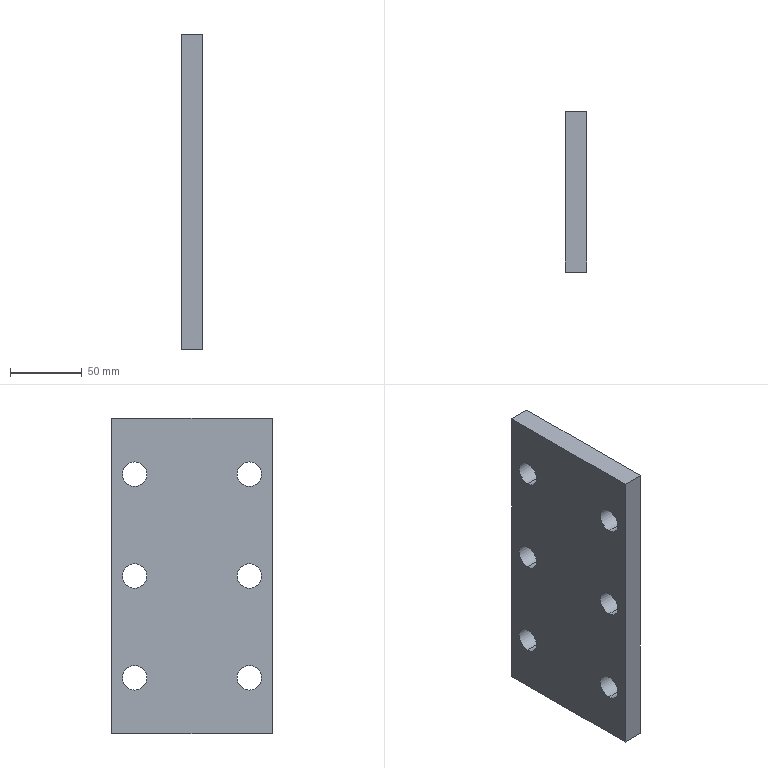Part | SolidWorks | features ICE 3, Extrusion 1 | 1 solid | 18 faces | box 15 x 112 x 220 mm | volume 349172 mm3 | cylinder 12 | plane 6 | commonest cylinder face diameters 17 x12
STEP:
#1=CARTESIAN_POINT('',(60.,-40.,101.5));
#2=VERTEX_POINT('',#1);
#3=CARTESIAN_POINT('',(60.,-40.,118.5));
#4=VERTEX_POINT('',#3);
#5=CARTESIAN_POINT('',(60.,-40.,110.));
#6=DIRECTION('',(-1.,0.,0.));
#7=DIRECTION('',(0.,1.,0.));
#8=AXIS2_PLACEMENT_3D('',#5,#6,#7);
#9=CIRCLE('',#8,8.5);
#10=EDGE_CURVE('',#2,#4,#9,.T.);
#11=ORIENTED_EDGE('',*,*,#10,.T.);
#12=CARTESIAN_POINT('',(75.,-40.,118.5));
#13=VERTEX_POINT('',#12);
#14=CARTESIAN_POINT('',(-45.001,-40.,118.5));
#15=DIRECTION('',(1.,0.,0.));
#16=VECTOR('',#15,1000.);
#17=LINE('',#14,#16);
#18=EDGE_CURVE('',#4,#13,#17,.T.);
#19=ORIENTED_EDGE('',*,*,#18,.T.);
#20=CARTESIAN_POINT('',(75.,-40.,101.5));
#21=VERTEX_POINT('',#20);
#22=CARTESIAN_POINT('',(75.,-40.,110.));
#23=DIRECTION('',(1.,0.,0.));
#24=DIRECTION('',(0.,0.,-1.));
#25=AXIS2_PLACEMENT_3D('',#22,#23,#24);
#26=CIRCLE('',#25,8.5);
#27=EDGE_CURVE('',#13,#21,#26,.T.);
#28=ORIENTED_EDGE('',*,*,#27,.T.);
#29=CARTESIAN_POINT('',(-45.001,-40.,101.5));
#30=DIRECTION('',(1.,0.,0.));
#31=VECTOR('',#30,1000.);
#32=LINE('',#29,#31);
#33=EDGE_CURVE('',#2,#21,#32,.T.);
#34=ORIENTED_EDGE('',*,*,#33,.F.);
#35=EDGE_LOOP('',(#11,#19,#28,#34));
#36=FACE_OUTER_BOUND('',#35,.T.);
#37=CARTESIAN_POINT('',(-45.001,-40.,110.));
#38=DIRECTION('',(1.,0.,0.));
#39=DIRECTION('',(0.,0.,-1.));
#40=AXIS2_PLACEMENT_3D('',#37,#38,#39);
#41=CYLINDRICAL_SURFACE('',#40,8.5);
#42=ADVANCED_FACE('',(#36),#41,.F.);
#43=CARTESIAN_POINT('',(60.,-40.,30.5));
#44=VERTEX_POINT('',#43);
#45=CARTESIAN_POINT('',(60.,-40.,47.5));
#46=VERTEX_POINT('',#45);
#47=CARTESIAN_POINT('',(60.,-40.,39.));
#48=DIRECTION('',(-1.,0.,0.));
#49=DIRECTION('',(0.,1.,0.));
#50=AXIS2_PLACEMENT_3D('',#47,#48,#49);
#51=CIRCLE('',#50,8.5);
#52=EDGE_CURVE('',#44,#46,#51,.T.);
#53=ORIENTED_EDGE('',*,*,#52,.T.);
#54=CARTESIAN_POINT('',(75.,-40.,47.5));
#55=VERTEX_POINT('',#54);
#56=CARTESIAN_POINT('',(-45.001,-40.,47.5));
#57=DIRECTION('',(1.,0.,0.));
#58=VECTOR('',#57,1000.);
#59=LINE('',#56,#58);
#60=EDGE_CURVE('',#46,#55,#59,.T.);
#61=ORIENTED_EDGE('',*,*,#60,.T.);
#62=CARTESIAN_POINT('',(75.,-40.,30.5));
#63=VERTEX_POINT('',#62);
#64=CARTESIAN_POINT('',(75.,-40.,39.));
#65=DIRECTION('',(1.,0.,0.));
#66=DIRECTION('',(0.,0.,-1.));
#67=AXIS2_PLACEMENT_3D('',#64,#65,#66);
#68=CIRCLE('',#67,8.5);
#69=EDGE_CURVE('',#55,#63,#68,.T.);
#70=ORIENTED_EDGE('',*,*,#69,.T.);
#71=CARTESIAN_POINT('',(-45.001,-40.,30.5));
#72=DIRECTION('',(1.,0.,0.));
#73=VECTOR('',#72,1000.);
#74=LINE('',#71,#73);
#75=EDGE_CURVE('',#44,#63,#74,.T.);
#76=ORIENTED_EDGE('',*,*,#75,.F.);
#77=EDGE_LOOP('',(#53,#61,#70,#76));
#78=FACE_OUTER_BOUND('',#77,.T.);
#79=CARTESIAN_POINT('',(-45.001,-40.,39.));
#80=DIRECTION('',(1.,0.,0.));
#81=DIRECTION('',(0.,0.,-1.));
#82=AXIS2_PLACEMENT_3D('',#79,#80,#81);
#83=CYLINDRICAL_SURFACE('',#82,8.5);
#84=ADVANCED_FACE('',(#78),#83,.F.);
#85=CARTESIAN_POINT('',(60.,-40.,172.5));
#86=VERTEX_POINT('',#85);
#87=CARTESIAN_POINT('',(60.,-40.,189.5));
#88=VERTEX_POINT('',#87);
#89=CARTESIAN_POINT('',(60.,-40.,181.));
#90=DIRECTION('',(-1.,0.,0.));
#91=DIRECTION('',(0.,1.,0.));
#92=AXIS2_PLACEMENT_3D('',#89,#90,#91);
#93=CIRCLE('',#92,8.5);
#94=EDGE_CURVE('',#86,#88,#93,.T.);
#95=ORIENTED_EDGE('',*,*,#94,.T.);
#96=CARTESIAN_POINT('',(75.,-40.,189.5));
#97=VERTEX_POINT('',#96);
#98=CARTESIAN_POINT('',(-45.001,-40.,189.5));
#99=DIRECTION('',(1.,0.,0.));
#100=VECTOR('',#99,1000.);
#101=LINE('',#98,#100);
#102=EDGE_CURVE('',#88,#97,#101,.T.);
#103=ORIENTED_EDGE('',*,*,#102,.T.);
#104=CARTESIAN_POINT('',(75.,-40.,172.5));
#105=VERTEX_POINT('',#104);
#106=CARTESIAN_POINT('',(75.,-40.,181.));
#107=DIRECTION('',(1.,0.,0.));
#108=DIRECTION('',(0.,0.,-1.));
#109=AXIS2_PLACEMENT_3D('',#106,#107,#108);
#110=CIRCLE('',#109,8.5);
#111=EDGE_CURVE('',#97,#105,#110,.T.);
#112=ORIENTED_EDGE('',*,*,#111,.T.);
#113=CARTESIAN_POINT('',(-45.001,-40.,172.5));
#114=DIRECTION('',(1.,0.,0.));
#115=VECTOR('',#114,1000.);
#116=LINE('',#113,#115);
#117=EDGE_CURVE('',#86,#105,#116,.T.);
#118=ORIENTED_EDGE('',*,*,#117,.F.);
#119=EDGE_LOOP('',(#95,#103,#112,#118));
#120=FACE_OUTER_BOUND('',#119,.T.);
#121=CARTESIAN_POINT('',(-45.001,-40.,181.));
#122=DIRECTION('',(1.,0.,0.));
#123=DIRECTION('',(0.,0.,-1.));
#124=AXIS2_PLACEMENT_3D('',#121,#122,#123);
#125=CYLINDRICAL_SURFACE('',#124,8.5);
#126=ADVANCED_FACE('',(#120),#125,.F.);
#127=CARTESIAN_POINT('',(60.,40.,172.5));
#128=VERTEX_POINT('',#127);
#129=CARTESIAN_POINT('',(60.,40.,189.5));
#130=VERTEX_POINT('',#129);
#131=CARTESIAN_POINT('',(60.,40.,181.));
#132=DIRECTION('',(-1.,0.,0.));
#133=DIRECTION('',(0.,1.,0.));
#134=AXIS2_PLACEMENT_3D('',#131,#132,#133);
#135=CIRCLE('',#134,8.5);
#136=EDGE_CURVE('',#128,#130,#135,.T.);
#137=ORIENTED_EDGE('',*,*,#136,.T.);
#138=CARTESIAN_POINT('',(75.,40.,189.5));
#139=VERTEX_POINT('',#138);
#140=CARTESIAN_POINT('',(-45.001,40.,189.5));
#141=DIRECTION('',(1.,0.,0.));
#142=VECTOR('',#141,1000.);
#143=LINE('',#140,#142);
#144=EDGE_CURVE('',#130,#139,#143,.T.);
#145=ORIENTED_EDGE('',*,*,#144,.T.);
#146=CARTESIAN_POINT('',(75.,40.,172.5));
#147=VERTEX_POINT('',#146);
#148=CARTESIAN_POINT('',(75.,40.,181.));
#149=DIRECTION('',(1.,0.,0.));
#150=DIRECTION('',(0.,0.,-1.));
#151=AXIS2_PLACEMENT_3D('',#148,#149,#150);
#152=CIRCLE('',#151,8.5);
#153=EDGE_CURVE('',#139,#147,#152,.T.);
#154=ORIENTED_EDGE('',*,*,#153,.T.);
#155=CARTESIAN_POINT('',(-45.001,40.,172.5));
#156=DIRECTION('',(1.,0.,0.));
#157=VECTOR('',#156,1000.);
#158=LINE('',#155,#157);
#159=EDGE_CURVE('',#128,#147,#158,.T.);
#160=ORIENTED_EDGE('',*,*,#159,.F.);
#161=EDGE_LOOP('',(#137,#145,#154,#160));
#162=FACE_OUTER_BOUND('',#161,.T.);
#163=CARTESIAN_POINT('',(-45.001,40.,181.));
#164=DIRECTION('',(1.,0.,0.));
#165=DIRECTION('',(0.,0.,-1.));
#166=AXIS2_PLACEMENT_3D('',#163,#164,#165);
#167=CYLINDRICAL_SURFACE('',#166,8.5);
#168=ADVANCED_FACE('',(#162),#167,.F.);
#169=CARTESIAN_POINT('',(60.,40.,101.5));
#170=VERTEX_POINT('',#169);
#171=CARTESIAN_POINT('',(60.,40.,118.5));
#172=VERTEX_POINT('',#171);
#173=CARTESIAN_POINT('',(60.,40.,110.));
#174=DIRECTION('',(-1.,0.,0.));
#175=DIRECTION('',(0.,1.,0.));
#176=AXIS2_PLACEMENT_3D('',#173,#174,#175);
#177=CIRCLE('',#176,8.5);
#178=EDGE_CURVE('',#170,#172,#177,.T.);
#179=ORIENTED_EDGE('',*,*,#178,.T.);
#180=CARTESIAN_POINT('',(75.,40.,118.5));
#181=VERTEX_POINT('',#180);
#182=CARTESIAN_POINT('',(-45.001,40.,118.5));
#183=DIRECTION('',(1.,0.,0.));
#184=VECTOR('',#183,1000.);
#185=LINE('',#182,#184);
#186=EDGE_CURVE('',#172,#181,#185,.T.);
#187=ORIENTED_EDGE('',*,*,#186,.T.);
#188=CARTESIAN_POINT('',(75.,40.,101.5));
#189=VERTEX_POINT('',#188);
#190=CARTESIAN_POINT('',(75.,40.,110.));
#191=DIRECTION('',(1.,0.,0.));
#192=DIRECTION('',(0.,0.,-1.));
#193=AXIS2_PLACEMENT_3D('',#190,#191,#192);
#194=CIRCLE('',#193,8.5);
#195=EDGE_CURVE('',#181,#189,#194,.T.);
#196=ORIENTED_EDGE('',*,*,#195,.T.);
#197=CARTESIAN_POINT('',(-45.001,40.,101.5));
#198=DIRECTION('',(1.,0.,0.));
#199=VECTOR('',#198,1000.);
#200=LINE('',#197,#199);
#201=EDGE_CURVE('',#170,#189,#200,.T.);
#202=ORIENTED_EDGE('',*,*,#201,.F.);
#203=EDGE_LOOP('',(#179,#187,#196,#202));
#204=FACE_OUTER_BOUND('',#203,.T.);
#205=CARTESIAN_POINT('',(-45.001,40.,110.));
#206=DIRECTION('',(1.,0.,0.));
#207=DIRECTION('',(0.,0.,-1.));
#208=AXIS2_PLACEMENT_3D('',#205,#206,#207);
#209=CYLINDRICAL_SURFACE('',#208,8.5);
#210=ADVANCED_FACE('',(#204),#209,.F.);
#211=CARTESIAN_POINT('',(60.,40.,30.5));
#212=VERTEX_POINT('',#211);
#213=CARTESIAN_POINT('',(60.,40.,47.5));
#214=VERTEX_POINT('',#213);
#215=CARTESIAN_POINT('',(60.,40.,39.));
#216=DIRECTION('',(-1.,0.,0.));
#217=DIRECTION('',(0.,1.,0.));
#218=AXIS2_PLACEMENT_3D('',#215,#216,#217);
#219=CIRCLE('',#218,8.5);
#220=EDGE_CURVE('',#212,#214,#219,.T.);
#221=ORIENTED_EDGE('',*,*,#220,.T.);
#222=CARTESIAN_POINT('',(75.,40.,47.5));
#223=VERTEX_POINT('',#222);
#224=CARTESIAN_POINT('',(-45.001,40.,47.5));
#225=DIRECTION('',(1.,0.,0.));
#226=VECTOR('',#225,1000.);
#227=LINE('',#224,#226);
#228=EDGE_CURVE('',#214,#223,#227,.T.);
#229=ORIENTED_EDGE('',*,*,#228,.T.);
#230=CARTESIAN_POINT('',(75.,40.,30.5));
#231=VERTEX_POINT('',#230);
#232=CARTESIAN_POINT('',(75.,40.,39.));
#233=DIRECTION('',(1.,0.,0.));
#234=DIRECTION('',(0.,0.,-1.));
#235=AXIS2_PLACEMENT_3D('',#232,#233,#234);
#236=CIRCLE('',#235,8.5);
#237=EDGE_CURVE('',#223,#231,#236,.T.);
#238=ORIENTED_EDGE('',*,*,#237,.T.);
#239=CARTESIAN_POINT('',(-45.001,40.,30.5));
#240=DIRECTION('',(1.,0.,0.));
#241=VECTOR('',#240,1000.);
#242=LINE('',#239,#241);
#243=EDGE_CURVE('',#212,#231,#242,.T.);
#244=ORIENTED_EDGE('',*,*,#243,.F.);
#245=EDGE_LOOP('',(#221,#229,#238,#244));
#246=FACE_OUTER_BOUND('',#245,.T.);
#247=CARTESIAN_POINT('',(-45.001,40.,39.));
#248=DIRECTION('',(1.,0.,0.));
#249=DIRECTION('',(0.,0.,-1.));
#250=AXIS2_PLACEMENT_3D('',#247,#248,#249);
#251=CYLINDRICAL_SURFACE('',#250,8.5);
#252=ADVANCED_FACE('',(#246),#251,.F.);
#253=CARTESIAN_POINT('',(75.,56.,220.));
#254=VERTEX_POINT('',#253);
#255=CARTESIAN_POINT('',(60.,56.,220.));
#256=VERTEX_POINT('',#255);
#257=CARTESIAN_POINT('',(75.,56.,220.));
#258=DIRECTION('',(-1.,0.,0.));
#259=VECTOR('',#258,1000.);
#260=LINE('',#257,#259);
#261=EDGE_CURVE('',#254,#256,#260,.T.);
#262=ORIENTED_EDGE('',*,*,#261,.T.);
#263=CARTESIAN_POINT('',(60.,-56.,220.));
#264=VERTEX_POINT('',#263);
#265=CARTESIAN_POINT('',(60.,-13.,220.));
#266=DIRECTION('',(0.,-1.,0.));
#267=VECTOR('',#266,1000.);
#268=LINE('',#265,#267);
#269=EDGE_CURVE('',#256,#264,#268,.T.);
#270=ORIENTED_EDGE('',*,*,#269,.T.);
#271=CARTESIAN_POINT('',(75.,-56.,220.));
#272=VERTEX_POINT('',#271);
#273=CARTESIAN_POINT('',(75.,-56.,220.));
#274=DIRECTION('',(1.,0.,0.));
#275=VECTOR('',#274,1000.);
#276=LINE('',#273,#275);
#277=EDGE_CURVE('',#264,#272,#276,.T.);
#278=ORIENTED_EDGE('',*,*,#277,.T.);
#279=CARTESIAN_POINT('',(75.,56.,220.));
#280=DIRECTION('',(0.,1.,0.));
#281=VECTOR('',#280,1000.);
#282=LINE('',#279,#281);
#283=EDGE_CURVE('',#272,#254,#282,.T.);
#284=ORIENTED_EDGE('',*,*,#283,.T.);
#285=EDGE_LOOP('',(#262,#270,#278,#284));
#286=FACE_OUTER_BOUND('',#285,.T.);
#287=CARTESIAN_POINT('',(0.,0.,220.));
#288=DIRECTION('',(0.,0.,1.));
#289=DIRECTION('',(1.,0.,0.));
#290=AXIS2_PLACEMENT_3D('',#287,#288,#289);
#291=PLANE('',#290);
#292=ADVANCED_FACE('',(#286),#291,.T.);
#293=CARTESIAN_POINT('',(60.,-56.,0.));
#294=VERTEX_POINT('',#293);
#295=CARTESIAN_POINT('',(75.,-56.,0.));
#296=VERTEX_POINT('',#295);
#297=CARTESIAN_POINT('',(75.,-56.,0.));
#298=DIRECTION('',(1.,0.,0.));
#299=VECTOR('',#298,1000.);
#300=LINE('',#297,#299);
#301=EDGE_CURVE('',#294,#296,#300,.T.);
#302=ORIENTED_EDGE('',*,*,#301,.F.);
#303=CARTESIAN_POINT('',(60.,56.,0.));
#304=VERTEX_POINT('',#303);
#305=CARTESIAN_POINT('',(60.,56.,0.));
#306=DIRECTION('',(0.,-1.,0.));
#307=VECTOR('',#306,1000.);
#308=LINE('',#305,#307);
#309=EDGE_CURVE('',#304,#294,#308,.T.);
#310=ORIENTED_EDGE('',*,*,#309,.F.);
#311=CARTESIAN_POINT('',(75.,56.,0.));
#312=VERTEX_POINT('',#311);
#313=CARTESIAN_POINT('',(75.,56.,0.));
#314=DIRECTION('',(-1.,0.,0.));
#315=VECTOR('',#314,1000.);
#316=LINE('',#313,#315);
#317=EDGE_CURVE('',#312,#304,#316,.T.);
#318=ORIENTED_EDGE('',*,*,#317,.F.);
#319=CARTESIAN_POINT('',(75.,56.,0.));
#320=DIRECTION('',(0.,1.,0.));
#321=VECTOR('',#320,1000.);
#322=LINE('',#319,#321);
#323=EDGE_CURVE('',#296,#312,#322,.T.);
#324=ORIENTED_EDGE('',*,*,#323,.F.);
#325=EDGE_LOOP('',(#302,#310,#318,#324));
#326=FACE_OUTER_BOUND('',#325,.T.);
#327=CARTESIAN_POINT('',(0.,0.,0.));
#328=DIRECTION('',(0.,0.,1.));
#329=DIRECTION('',(1.,0.,0.));
#330=AXIS2_PLACEMENT_3D('',#327,#328,#329);
#331=PLANE('',#330);
#332=ADVANCED_FACE('',(#326),#331,.F.);
#333=ORIENTED_EDGE('',*,*,#301,.T.);
#334=CARTESIAN_POINT('',(75.,-56.,220.));
#335=DIRECTION('',(0.,0.,-1.));
#336=VECTOR('',#335,1000.);
#337=LINE('',#334,#336);
#338=EDGE_CURVE('',#272,#296,#337,.T.);
#339=ORIENTED_EDGE('',*,*,#338,.F.);
#340=ORIENTED_EDGE('',*,*,#277,.F.);
#341=CARTESIAN_POINT('',(60.,-56.,220.));
#342=DIRECTION('',(0.,0.,-1.));
#343=VECTOR('',#342,1000.);
#344=LINE('',#341,#343);
#345=EDGE_CURVE('',#264,#294,#344,.T.);
#346=ORIENTED_EDGE('',*,*,#345,.T.);
#347=EDGE_LOOP('',(#333,#339,#340,#346));
#348=FACE_OUTER_BOUND('',#347,.T.);
#349=CARTESIAN_POINT('',(75.,-56.,220.));
#350=DIRECTION('',(0.,1.,0.));
#351=DIRECTION('',(0.,0.,1.));
#352=AXIS2_PLACEMENT_3D('',#349,#350,#351);
#353=PLANE('',#352);
#354=ADVANCED_FACE('',(#348),#353,.F.);
#355=CARTESIAN_POINT('',(75.,40.,181.));
#356=DIRECTION('',(1.,0.,0.));
#357=DIRECTION('',(0.,0.,-1.));
#358=AXIS2_PLACEMENT_3D('',#355,#356,#357);
#359=CIRCLE('',#358,8.5);
#360=EDGE_CURVE('',#147,#139,#359,.T.);
#361=ORIENTED_EDGE('',*,*,#360,.F.);
#362=ORIENTED_EDGE('',*,*,#153,.F.);
#363=EDGE_LOOP('',(#361,#362));
#364=FACE_BOUND('',#363,.T.);
#365=CARTESIAN_POINT('',(75.,40.,110.));
#366=DIRECTION('',(1.,0.,0.));
#367=DIRECTION('',(0.,0.,-1.));
#368=AXIS2_PLACEMENT_3D('',#365,#366,#367);
#369=CIRCLE('',#368,8.5);
#370=EDGE_CURVE('',#189,#181,#369,.T.);
#371=ORIENTED_EDGE('',*,*,#370,.F.);
#372=ORIENTED_EDGE('',*,*,#195,.F.);
#373=EDGE_LOOP('',(#371,#372));
#374=FACE_BOUND('',#373,.T.);
#375=CARTESIAN_POINT('',(75.,-40.,110.));
#376=DIRECTION('',(1.,0.,0.));
#377=DIRECTION('',(0.,0.,-1.));
#378=AXIS2_PLACEMENT_3D('',#375,#376,#377);
#379=CIRCLE('',#378,8.5);
#380=EDGE_CURVE('',#21,#13,#379,.T.);
#381=ORIENTED_EDGE('',*,*,#380,.F.);
#382=ORIENTED_EDGE('',*,*,#27,.F.);
#383=EDGE_LOOP('',(#381,#382));
#384=FACE_BOUND('',#383,.T.);
#385=CARTESIAN_POINT('',(75.,-40.,39.));
#386=DIRECTION('',(1.,0.,0.));
#387=DIRECTION('',(0.,0.,-1.));
#388=AXIS2_PLACEMENT_3D('',#385,#386,#387);
#389=CIRCLE('',#388,8.5);
#390=EDGE_CURVE('',#63,#55,#389,.T.);
#391=ORIENTED_EDGE('',*,*,#390,.F.);
#392=ORIENTED_EDGE('',*,*,#69,.F.);
#393=EDGE_LOOP('',(#391,#392));
#394=FACE_BOUND('',#393,.T.);
#395=CARTESIAN_POINT('',(75.,40.,39.));
#396=DIRECTION('',(1.,0.,0.));
#397=DIRECTION('',(0.,0.,-1.));
#398=AXIS2_PLACEMENT_3D('',#395,#396,#397);
#399=CIRCLE('',#398,8.5);
#400=EDGE_CURVE('',#231,#223,#399,.T.);
#401=ORIENTED_EDGE('',*,*,#400,.F.);
#402=ORIENTED_EDGE('',*,*,#237,.F.);
#403=EDGE_LOOP('',(#401,#402));
#404=FACE_BOUND('',#403,.T.);
#405=CARTESIAN_POINT('',(75.,-40.,181.));
#406=DIRECTION('',(1.,0.,0.));
#407=DIRECTION('',(0.,0.,-1.));
#408=AXIS2_PLACEMENT_3D('',#405,#406,#407);
#409=CIRCLE('',#408,8.5);
#410=EDGE_CURVE('',#105,#97,#409,.T.);
#411=ORIENTED_EDGE('',*,*,#410,.F.);
#412=ORIENTED_EDGE('',*,*,#111,.F.);
#413=EDGE_LOOP('',(#411,#412));
#414=FACE_BOUND('',#413,.T.);
#415=ORIENTED_EDGE('',*,*,#323,.T.);
#416=CARTESIAN_POINT('',(75.,56.,220.));
#417=DIRECTION('',(0.,0.,-1.));
#418=VECTOR('',#417,1000.);
#419=LINE('',#416,#418);
#420=EDGE_CURVE('',#254,#312,#419,.T.);
#421=ORIENTED_EDGE('',*,*,#420,.F.);
#422=ORIENTED_EDGE('',*,*,#283,.F.);
#423=ORIENTED_EDGE('',*,*,#338,.T.);
#424=EDGE_LOOP('',(#415,#421,#422,#423));
#425=FACE_OUTER_BOUND('',#424,.T.);
#426=CARTESIAN_POINT('',(75.,56.,220.));
#427=DIRECTION('',(-1.,0.,0.));
#428=DIRECTION('',(0.,0.,1.));
#429=AXIS2_PLACEMENT_3D('',#426,#427,#428);
#430=PLANE('',#429);
#431=ADVANCED_FACE('',(#364,#374,#384,#394,#404,#414,#425),#430,.F.);
#432=ORIENTED_EDGE('',*,*,#317,.T.);
#433=CARTESIAN_POINT('',(60.,56.,220.));
#434=DIRECTION('',(0.,0.,-1.));
#435=VECTOR('',#434,1000.);
#436=LINE('',#433,#435);
#437=EDGE_CURVE('',#256,#304,#436,.T.);
#438=ORIENTED_EDGE('',*,*,#437,.F.);
#439=ORIENTED_EDGE('',*,*,#261,.F.);
#440=ORIENTED_EDGE('',*,*,#420,.T.);
#441=EDGE_LOOP('',(#432,#438,#439,#440));
#442=FACE_OUTER_BOUND('',#441,.T.);
#443=CARTESIAN_POINT('',(75.,56.,220.));
#444=DIRECTION('',(0.,-1.,0.));
#445=DIRECTION('',(0.,0.,-1.));
#446=AXIS2_PLACEMENT_3D('',#443,#444,#445);
#447=PLANE('',#446);
#448=ADVANCED_FACE('',(#442),#447,.F.);
#449=ORIENTED_EDGE('',*,*,#136,.F.);
#450=CARTESIAN_POINT('',(60.,40.,181.));
#451=DIRECTION('',(-1.,0.,0.));
#452=DIRECTION('',(0.,1.,0.));
#453=AXIS2_PLACEMENT_3D('',#450,#451,#452);
#454=CIRCLE('',#453,8.5);
#455=EDGE_CURVE('',#130,#128,#454,.T.);
#456=ORIENTED_EDGE('',*,*,#455,.F.);
#457=EDGE_LOOP('',(#449,#456));
#458=FACE_BOUND('',#457,.T.);
#459=ORIENTED_EDGE('',*,*,#178,.F.);
#460=CARTESIAN_POINT('',(60.,40.,110.));
#461=DIRECTION('',(-1.,0.,0.));
#462=DIRECTION('',(0.,1.,0.));
#463=AXIS2_PLACEMENT_3D('',#460,#461,#462);
#464=CIRCLE('',#463,8.5);
#465=EDGE_CURVE('',#172,#170,#464,.T.);
#466=ORIENTED_EDGE('',*,*,#465,.F.);
#467=EDGE_LOOP('',(#459,#466));
#468=FACE_BOUND('',#467,.T.);
#469=ORIENTED_EDGE('',*,*,#220,.F.);
#470=CARTESIAN_POINT('',(60.,40.,39.));
#471=DIRECTION('',(-1.,0.,0.));
#472=DIRECTION('',(0.,1.,0.));
#473=AXIS2_PLACEMENT_3D('',#470,#471,#472);
#474=CIRCLE('',#473,8.5);
#475=EDGE_CURVE('',#214,#212,#474,.T.);
#476=ORIENTED_EDGE('',*,*,#475,.F.);
#477=EDGE_LOOP('',(#469,#476));
#478=FACE_BOUND('',#477,.T.);
#479=ORIENTED_EDGE('',*,*,#309,.T.);
#480=ORIENTED_EDGE('',*,*,#345,.F.);
#481=ORIENTED_EDGE('',*,*,#269,.F.);
#482=ORIENTED_EDGE('',*,*,#437,.T.);
#483=EDGE_LOOP('',(#479,#480,#481,#482));
#484=FACE_OUTER_BOUND('',#483,.T.);
#485=ORIENTED_EDGE('',*,*,#10,.F.);
#486=CARTESIAN_POINT('',(60.,-40.,110.));
#487=DIRECTION('',(-1.,0.,0.));
#488=DIRECTION('',(0.,1.,0.));
#489=AXIS2_PLACEMENT_3D('',#486,#487,#488);
#490=CIRCLE('',#489,8.5);
#491=EDGE_CURVE('',#4,#2,#490,.T.);
#492=ORIENTED_EDGE('',*,*,#491,.F.);
#493=EDGE_LOOP('',(#485,#492));
#494=FACE_BOUND('',#493,.T.);
#495=ORIENTED_EDGE('',*,*,#52,.F.);
#496=CARTESIAN_POINT('',(60.,-40.,39.));
#497=DIRECTION('',(-1.,0.,0.));
#498=DIRECTION('',(0.,1.,0.));
#499=AXIS2_PLACEMENT_3D('',#496,#497,#498);
#500=CIRCLE('',#499,8.5);
#501=EDGE_CURVE('',#46,#44,#500,.T.);
#502=ORIENTED_EDGE('',*,*,#501,.F.);
#503=EDGE_LOOP('',(#495,#502));
#504=FACE_BOUND('',#503,.T.);
#505=ORIENTED_EDGE('',*,*,#94,.F.);
#506=CARTESIAN_POINT('',(60.,-40.,181.));
#507=DIRECTION('',(-1.,0.,0.));
#508=DIRECTION('',(0.,1.,0.));
#509=AXIS2_PLACEMENT_3D('',#506,#507,#508);
#510=CIRCLE('',#509,8.5);
#511=EDGE_CURVE('',#88,#86,#510,.T.);
#512=ORIENTED_EDGE('',*,*,#511,.F.);
#513=EDGE_LOOP('',(#505,#512));
#514=FACE_BOUND('',#513,.T.);
#515=CARTESIAN_POINT('',(60.,56.,220.));
#516=DIRECTION('',(1.,0.,0.));
#517=DIRECTION('',(0.,1.,0.));
#518=AXIS2_PLACEMENT_3D('',#515,#516,#517);
#519=PLANE('',#518);
#520=ADVANCED_FACE('',(#458,#468,#478,#484,#494,#504,#514),#519,.F.);
#521=ORIENTED_EDGE('',*,*,#228,.F.);
#522=ORIENTED_EDGE('',*,*,#475,.T.);
#523=ORIENTED_EDGE('',*,*,#243,.T.);
#524=ORIENTED_EDGE('',*,*,#400,.T.);
#525=EDGE_LOOP('',(#521,#522,#523,#524));
#526=FACE_OUTER_BOUND('',#525,.T.);
#527=CARTESIAN_POINT('',(-45.001,40.,39.));
#528=DIRECTION('',(1.,0.,0.));
#529=DIRECTION('',(0.,0.,-1.));
#530=AXIS2_PLACEMENT_3D('',#527,#528,#529);
#531=CYLINDRICAL_SURFACE('',#530,8.5);
#532=ADVANCED_FACE('',(#526),#531,.F.);
#533=ORIENTED_EDGE('',*,*,#186,.F.);
#534=ORIENTED_EDGE('',*,*,#465,.T.);
#535=ORIENTED_EDGE('',*,*,#201,.T.);
#536=ORIENTED_EDGE('',*,*,#370,.T.);
#537=EDGE_LOOP('',(#533,#534,#535,#536));
#538=FACE_OUTER_BOUND('',#537,.T.);
#539=CARTESIAN_POINT('',(-45.001,40.,110.));
#540=DIRECTION('',(1.,0.,0.));
#541=DIRECTION('',(0.,0.,-1.));
#542=AXIS2_PLACEMENT_3D('',#539,#540,#541);
#543=CYLINDRICAL_SURFACE('',#542,8.5);
#544=ADVANCED_FACE('',(#538),#543,.F.);
#545=ORIENTED_EDGE('',*,*,#144,.F.);
#546=ORIENTED_EDGE('',*,*,#455,.T.);
#547=ORIENTED_EDGE('',*,*,#159,.T.);
#548=ORIENTED_EDGE('',*,*,#360,.T.);
#549=EDGE_LOOP('',(#545,#546,#547,#548));
#550=FACE_OUTER_BOUND('',#549,.T.);
#551=CARTESIAN_POINT('',(-45.001,40.,181.));
#552=DIRECTION('',(1.,0.,0.));
#553=DIRECTION('',(0.,0.,-1.));
#554=AXIS2_PLACEMENT_3D('',#551,#552,#553);
#555=CYLINDRICAL_SURFACE('',#554,8.5);
#556=ADVANCED_FACE('',(#550),#555,.F.);
#557=ORIENTED_EDGE('',*,*,#102,.F.);
#558=ORIENTED_EDGE('',*,*,#511,.T.);
#559=ORIENTED_EDGE('',*,*,#117,.T.);
#560=ORIENTED_EDGE('',*,*,#410,.T.);
#561=EDGE_LOOP('',(#557,#558,#559,#560));
#562=FACE_OUTER_BOUND('',#561,.T.);
#563=CARTESIAN_POINT('',(-45.001,-40.,181.));
#564=DIRECTION('',(1.,0.,0.));
#565=DIRECTION('',(0.,0.,-1.));
#566=AXIS2_PLACEMENT_3D('',#563,#564,#565);
#567=CYLINDRICAL_SURFACE('',#566,8.5);
#568=ADVANCED_FACE('',(#562),#567,.F.);
#569=ORIENTED_EDGE('',*,*,#60,.F.);
#570=ORIENTED_EDGE('',*,*,#501,.T.);
#571=ORIENTED_EDGE('',*,*,#75,.T.);
#572=ORIENTED_EDGE('',*,*,#390,.T.);
#573=EDGE_LOOP('',(#569,#570,#571,#572));
#574=FACE_OUTER_BOUND('',#573,.T.);
#575=CARTESIAN_POINT('',(-45.001,-40.,39.));
#576=DIRECTION('',(1.,0.,0.));
#577=DIRECTION('',(0.,0.,-1.));
#578=AXIS2_PLACEMENT_3D('',#575,#576,#577);
#579=CYLINDRICAL_SURFACE('',#578,8.5);
#580=ADVANCED_FACE('',(#574),#579,.F.);
#581=ORIENTED_EDGE('',*,*,#18,.F.);
#582=ORIENTED_EDGE('',*,*,#491,.T.);
#583=ORIENTED_EDGE('',*,*,#33,.T.);
#584=ORIENTED_EDGE('',*,*,#380,.T.);
#585=EDGE_LOOP('',(#581,#582,#583,#584));
#586=FACE_OUTER_BOUND('',#585,.T.);
#587=CARTESIAN_POINT('',(-45.001,-40.,110.));
#588=DIRECTION('',(1.,0.,0.));
#589=DIRECTION('',(0.,0.,-1.));
#590=AXIS2_PLACEMENT_3D('',#587,#588,#589);
#591=CYLINDRICAL_SURFACE('',#590,8.5);
#592=ADVANCED_FACE('',(#586),#591,.F.);
#593=CLOSED_SHELL('',(#42,#84,#126,#168,#210,#252,#292,#332,#354,#431,#448,#520,#532,#544,#556,#568,#580,#592));
#594=MANIFOLD_SOLID_BREP('',#593);
#595=CARTESIAN_POINT('',(0.,0.,0.));
#596=DIRECTION('',(0.,0.,1.));
#597=DIRECTION('',(1.,0.,0.));
#598=AXIS2_PLACEMENT_3D('',#595,#596,#597);
#599=(LENGTH_UNIT()NAMED_UNIT(*)SI_UNIT(.MILLI.,.METRE.));
#600=UNCERTAINTY_MEASURE_WITH_UNIT(LENGTH_MEASURE(0.00001),#599,'','');
#601=(NAMED_UNIT(*)PLANE_ANGLE_UNIT()SI_UNIT($,.RADIAN.));
#602=(NAMED_UNIT(*)SI_UNIT($,.STERADIAN.)SOLID_ANGLE_UNIT());
#603=(GEOMETRIC_REPRESENTATION_CONTEXT(3)GLOBAL_UNCERTAINTY_ASSIGNED_CONTEXT((#600))GLOBAL_UNIT_ASSIGNED_CONTEXT((#599,#601,#602))REPRESENTATION_CONTEXT('',''));
#604=ADVANCED_BREP_SHAPE_REPRESENTATION('',(#594,#598),#603);